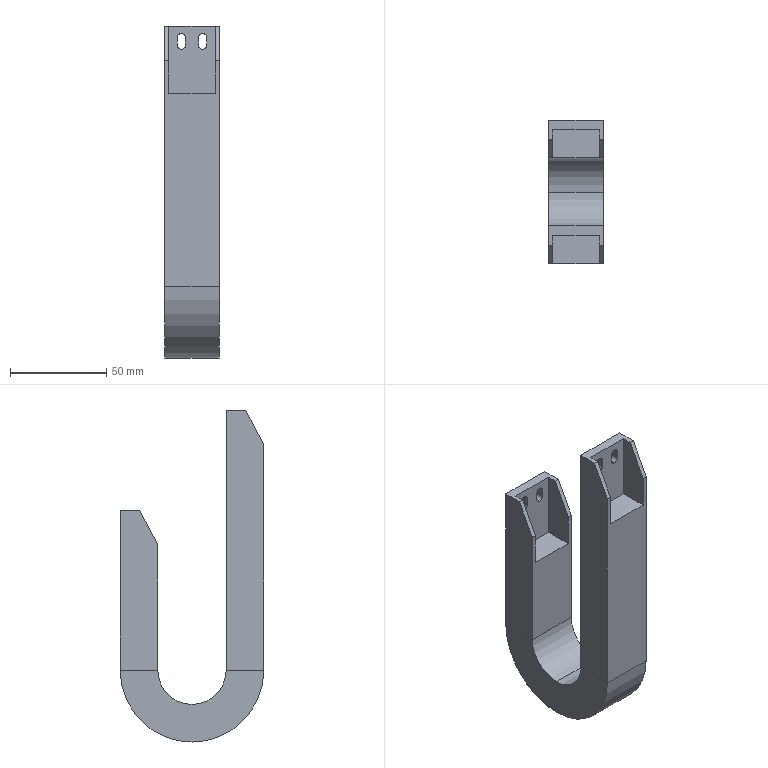Part | STEP file | JFLO drag chain 15.20B, bend radius R28 | 1 solid | 48 faces | box 28.5 x 74.5 x 172.25 mm | volume 143432 mm3 | plane 32 | cylinder 16 | commonest cylinder face diameters 4.2 x12 35.5 x2 74.5 x2